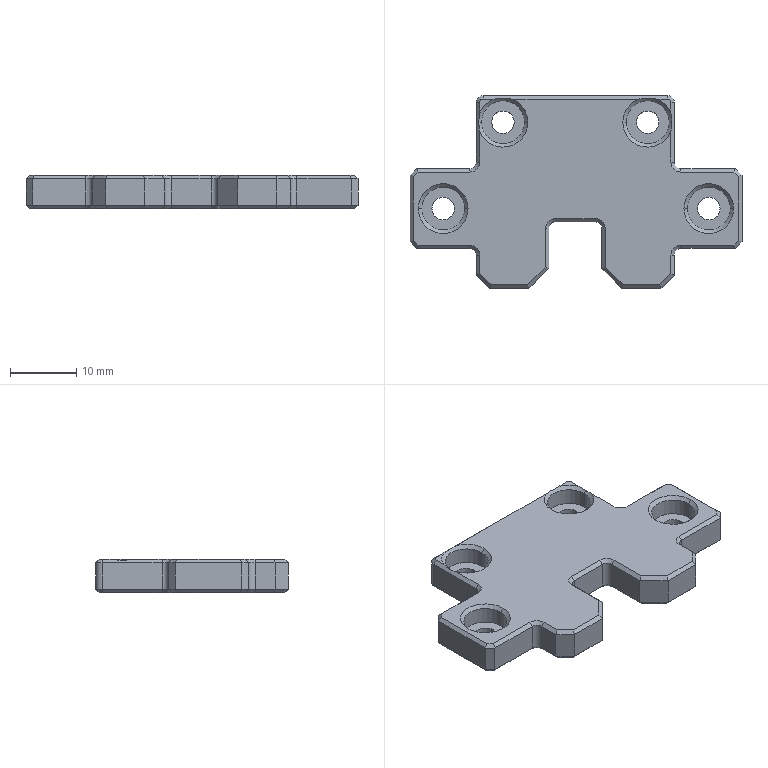Part | SolidWorks | features Chamfer 1, Extrusion 1, HoleWzd 1 | 1 solid | 136 faces | box 50 x 29 x 5 mm | volume 4534 mm3 | plane 80 | cone 32 | cylinder 24 | commonest cylinder face diameters 2 x8 3.4 x8 6.5 x8